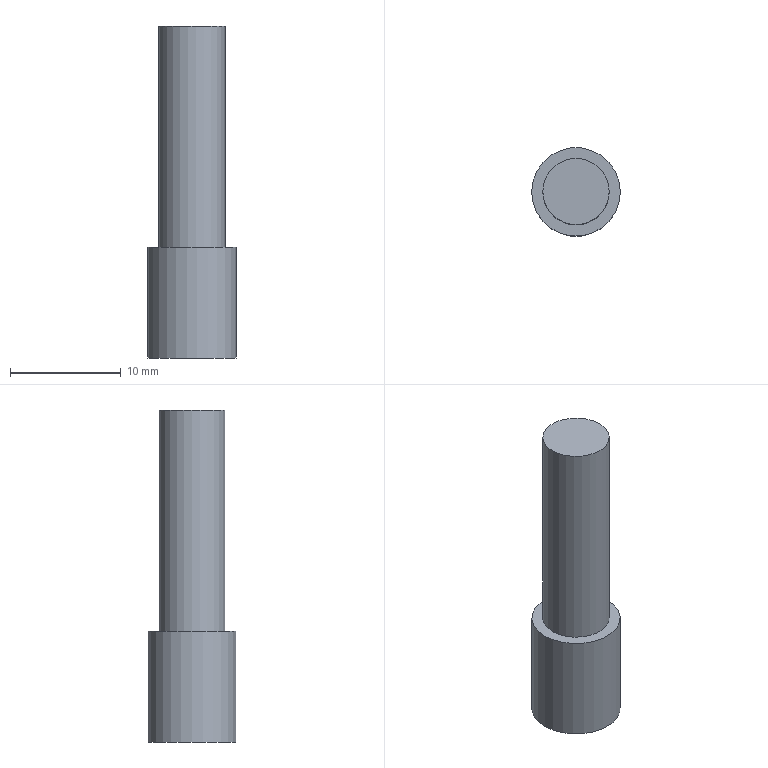Part | NX | features solid 2 | 1 solid | 5 faces | box 8 x 8 x 30 mm | volume 1068 mm3 | plane 3 | cylinder 2 | commonest cylinder face diameters 6 x1 8 x1
STEP:
#1=CARTESIAN_POINT('',(-70.,72.,-20.));
#2=VERTEX_POINT('',#1);
#3=CARTESIAN_POINT('',(-67.,72.,-20.));
#4=DIRECTION('',(0.,0.,-1.));
#5=DIRECTION('',(-1.,0.,0.));
#6=AXIS2_PLACEMENT_3D('',#3,#4,#5);
#7=CIRCLE('',#6,3.);
#8=EDGE_CURVE('',#2,#2,#7,.T.);
#9=ORIENTED_EDGE('',*,*,#8,.T.);
#10=EDGE_LOOP('',(#9));
#11=FACE_BOUND('',#10,.T.);
#12=CARTESIAN_POINT('',(-70.,72.,-40.));
#13=VERTEX_POINT('',#12);
#14=CARTESIAN_POINT('',(-67.,72.,-40.));
#15=DIRECTION('',(0.,0.,-1.));
#16=DIRECTION('',(-1.,0.,0.));
#17=AXIS2_PLACEMENT_3D('',#14,#15,#16);
#18=CIRCLE('',#17,3.);
#19=EDGE_CURVE('',#13,#13,#18,.T.);
#20=ORIENTED_EDGE('',*,*,#19,.F.);
#21=EDGE_LOOP('',(#20));
#22=FACE_BOUND('',#21,.T.);
#23=CARTESIAN_POINT('',(-67.,72.,-35.));
#24=DIRECTION('',(0.,0.,1.));
#25=DIRECTION('',(-1.,0.,0.));
#26=AXIS2_PLACEMENT_3D('',#23,#24,#25);
#27=CYLINDRICAL_SURFACE('',#26,3.);
#28=ADVANCED_FACE('',(#11,#22),#27,.T.);
#29=ORIENTED_EDGE('',*,*,#8,.F.);
#30=EDGE_LOOP('',(#29));
#31=FACE_BOUND('',#30,.T.);
#32=CARTESIAN_POINT('',(-67.,72.,-20.));
#33=DIRECTION('',(0.,0.,1.));
#34=DIRECTION('',(-1.,0.,0.));
#35=AXIS2_PLACEMENT_3D('',#32,#33,#34);
#36=PLANE('',#35);
#37=ADVANCED_FACE('',(#31),#36,.T.);
#38=CARTESIAN_POINT('',(-71.,72.,-40.));
#39=VERTEX_POINT('',#38);
#40=CARTESIAN_POINT('',(-67.,72.,-40.));
#41=DIRECTION('',(0.,0.,-1.));
#42=DIRECTION('',(-1.,0.,0.));
#43=AXIS2_PLACEMENT_3D('',#40,#41,#42);
#44=CIRCLE('',#43,4.);
#45=EDGE_CURVE('',#39,#39,#44,.F.);
#46=ORIENTED_EDGE('',*,*,#45,.F.);
#47=EDGE_LOOP('',(#46));
#48=FACE_BOUND('',#47,.T.);
#49=CARTESIAN_POINT('',(-63.,72.,-50.));
#50=VERTEX_POINT('',#49);
#51=CARTESIAN_POINT('',(-67.,72.,-50.));
#52=DIRECTION('',(0.,0.,1.));
#53=DIRECTION('',(1.,0.,0.));
#54=AXIS2_PLACEMENT_3D('',#51,#52,#53);
#55=CIRCLE('',#54,4.);
#56=EDGE_CURVE('',#50,#50,#55,.T.);
#57=ORIENTED_EDGE('',*,*,#56,.T.);
#58=EDGE_LOOP('',(#57));
#59=FACE_BOUND('',#58,.T.);
#60=CARTESIAN_POINT('',(-67.,72.,-38.));
#61=DIRECTION('',(0.,0.,-1.));
#62=DIRECTION('',(1.,0.,0.));
#63=AXIS2_PLACEMENT_3D('',#60,#61,#62);
#64=CYLINDRICAL_SURFACE('',#63,4.);
#65=ADVANCED_FACE('',(#48,#59),#64,.T.);
#66=ORIENTED_EDGE('',*,*,#19,.T.);
#67=EDGE_LOOP('',(#66));
#68=FACE_BOUND('',#67,.T.);
#69=ORIENTED_EDGE('',*,*,#45,.T.);
#70=EDGE_LOOP('',(#69));
#71=FACE_BOUND('',#70,.T.);
#72=CARTESIAN_POINT('',(-67.,72.,-40.));
#73=DIRECTION('',(0.,0.,-1.));
#74=DIRECTION('',(1.,0.,0.));
#75=AXIS2_PLACEMENT_3D('',#72,#73,#74);
#76=PLANE('',#75);
#77=ADVANCED_FACE('',(#68,#71),#76,.F.);
#78=ORIENTED_EDGE('',*,*,#56,.F.);
#79=EDGE_LOOP('',(#78));
#80=FACE_BOUND('',#79,.T.);
#81=CARTESIAN_POINT('',(-8.802,-49.836,-50.));
#82=DIRECTION('',(0.,0.,1.));
#83=DIRECTION('',(1.,0.,0.));
#84=AXIS2_PLACEMENT_3D('',#81,#82,#83);
#85=PLANE('',#84);
#86=ADVANCED_FACE('',(#80),#85,.F.);
#87=CLOSED_SHELL('',(#28,#37,#65,#77,#86));
#88=MANIFOLD_SOLID_BREP('',#87);
#89=(LENGTH_UNIT()NAMED_UNIT(*)SI_UNIT(.MILLI.,.METRE.));
#90=UNCERTAINTY_MEASURE_WITH_UNIT(LENGTH_MEASURE(0.00001),#89,'','');
#91=(NAMED_UNIT(*)PLANE_ANGLE_UNIT()SI_UNIT($,.RADIAN.));
#92=(NAMED_UNIT(*)SI_UNIT($,.STERADIAN.)SOLID_ANGLE_UNIT());
#93=(GEOMETRIC_REPRESENTATION_CONTEXT(3)GLOBAL_UNCERTAINTY_ASSIGNED_CONTEXT((#90))GLOBAL_UNIT_ASSIGNED_CONTEXT((#89,#91,#92))REPRESENTATION_CONTEXT('',''));
#94=ADVANCED_BREP_SHAPE_REPRESENTATION('',(#88),#93);